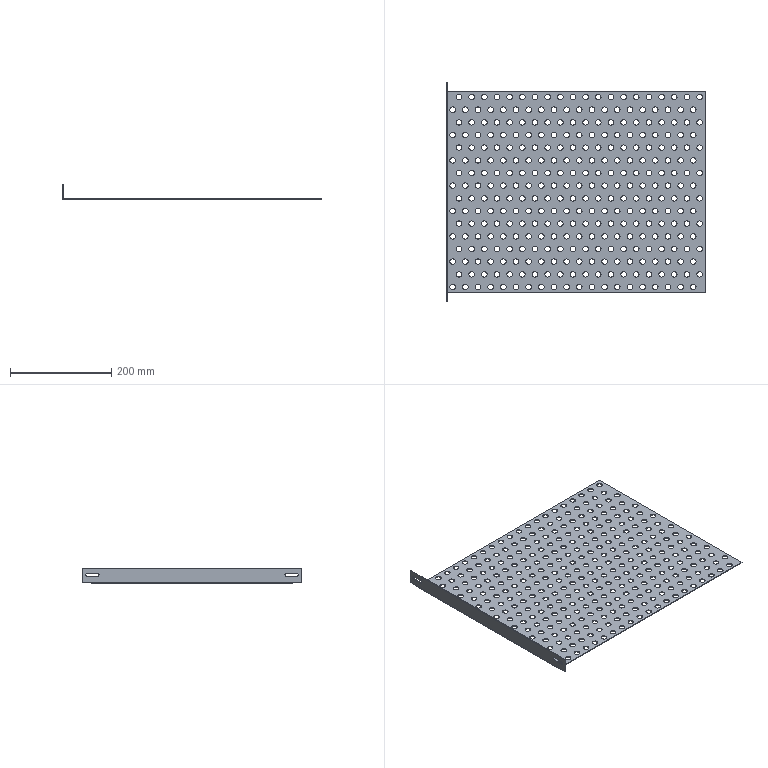Part | STEP file | part 153^evaporator 408 by COMPANY_A | 1 solid | 666 faces | box 512 x 433 x 30.095 mm | volume 277126 mm3 | cylinder 646 | plane 20 | commonest cylinder face diameters 11 x640 6 x4 0.2 x1 3.2 x1